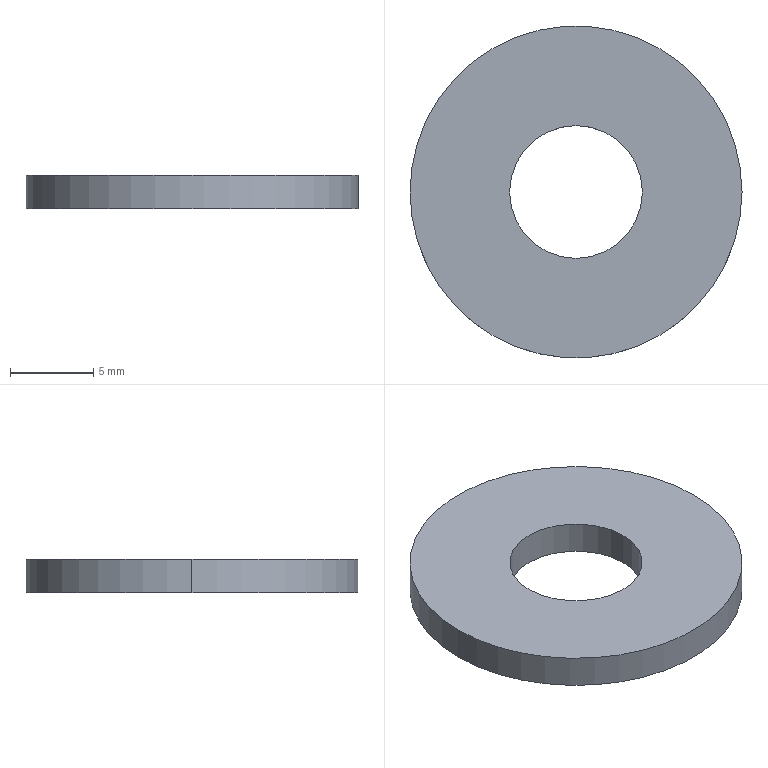Part | SolidWorks | features Extrusion 1 | 1 solid | 6 faces | box 20 x 20 x 2 mm | volume 527.788 mm3 | cylinder 4 | plane 2 | commonest cylinder face diameters 8 x2 20 x2
STEP:
#1=CARTESIAN_POINT('',(-4.,0.,2.));
#2=VERTEX_POINT('',#1);
#3=CARTESIAN_POINT('',(4.,0.,2.));
#4=VERTEX_POINT('',#3);
#5=CARTESIAN_POINT('',(0.,0.,2.));
#6=DIRECTION('',(0.,0.,1.));
#7=DIRECTION('',(1.,0.,0.));
#8=AXIS2_PLACEMENT_3D('',#5,#6,#7);
#9=CIRCLE('',#8,4.);
#10=EDGE_CURVE('',#2,#4,#9,.T.);
#11=ORIENTED_EDGE('',*,*,#10,.T.);
#12=CARTESIAN_POINT('',(4.,0.,0.));
#13=VERTEX_POINT('',#12);
#14=CARTESIAN_POINT('',(4.,0.,2.));
#15=DIRECTION('',(0.,0.,-1.));
#16=VECTOR('',#15,1000.);
#17=LINE('',#14,#16);
#18=EDGE_CURVE('',#4,#13,#17,.T.);
#19=ORIENTED_EDGE('',*,*,#18,.T.);
#20=CARTESIAN_POINT('',(-4.,0.,0.));
#21=VERTEX_POINT('',#20);
#22=CARTESIAN_POINT('',(0.,0.,0.));
#23=DIRECTION('',(0.,0.,1.));
#24=DIRECTION('',(1.,0.,0.));
#25=AXIS2_PLACEMENT_3D('',#22,#23,#24);
#26=CIRCLE('',#25,4.);
#27=EDGE_CURVE('',#21,#13,#26,.T.);
#28=ORIENTED_EDGE('',*,*,#27,.F.);
#29=CARTESIAN_POINT('',(-4.,0.,2.));
#30=DIRECTION('',(0.,0.,-1.));
#31=VECTOR('',#30,1000.);
#32=LINE('',#29,#31);
#33=EDGE_CURVE('',#2,#21,#32,.T.);
#34=ORIENTED_EDGE('',*,*,#33,.F.);
#35=EDGE_LOOP('',(#11,#19,#28,#34));
#36=FACE_OUTER_BOUND('',#35,.T.);
#37=CARTESIAN_POINT('',(0.,0.,2.));
#38=DIRECTION('',(0.,0.,-1.));
#39=DIRECTION('',(-1.,0.,0.));
#40=AXIS2_PLACEMENT_3D('',#37,#38,#39);
#41=CYLINDRICAL_SURFACE('',#40,4.);
#42=ADVANCED_FACE('',(#36),#41,.F.);
#43=CARTESIAN_POINT('',(10.,0.,2.));
#44=VERTEX_POINT('',#43);
#45=CARTESIAN_POINT('',(-10.,0.,2.));
#46=VERTEX_POINT('',#45);
#47=CARTESIAN_POINT('',(0.,0.,2.));
#48=DIRECTION('',(0.,0.,1.));
#49=DIRECTION('',(1.,0.,0.));
#50=AXIS2_PLACEMENT_3D('',#47,#48,#49);
#51=CIRCLE('',#50,10.);
#52=EDGE_CURVE('',#44,#46,#51,.T.);
#53=ORIENTED_EDGE('',*,*,#52,.F.);
#54=CARTESIAN_POINT('',(10.,0.,0.));
#55=VERTEX_POINT('',#54);
#56=CARTESIAN_POINT('',(10.,0.,2.));
#57=DIRECTION('',(0.,0.,-1.));
#58=VECTOR('',#57,1000.);
#59=LINE('',#56,#58);
#60=EDGE_CURVE('',#44,#55,#59,.T.);
#61=ORIENTED_EDGE('',*,*,#60,.T.);
#62=CARTESIAN_POINT('',(-10.,0.,0.));
#63=VERTEX_POINT('',#62);
#64=CARTESIAN_POINT('',(0.,0.,0.));
#65=DIRECTION('',(0.,0.,1.));
#66=DIRECTION('',(1.,0.,0.));
#67=AXIS2_PLACEMENT_3D('',#64,#65,#66);
#68=CIRCLE('',#67,10.);
#69=EDGE_CURVE('',#55,#63,#68,.T.);
#70=ORIENTED_EDGE('',*,*,#69,.T.);
#71=CARTESIAN_POINT('',(-10.,0.,2.));
#72=DIRECTION('',(0.,0.,-1.));
#73=VECTOR('',#72,1000.);
#74=LINE('',#71,#73);
#75=EDGE_CURVE('',#46,#63,#74,.T.);
#76=ORIENTED_EDGE('',*,*,#75,.F.);
#77=EDGE_LOOP('',(#53,#61,#70,#76));
#78=FACE_OUTER_BOUND('',#77,.T.);
#79=CARTESIAN_POINT('',(0.,0.,2.));
#80=DIRECTION('',(0.,0.,-1.));
#81=DIRECTION('',(-1.,0.,0.));
#82=AXIS2_PLACEMENT_3D('',#79,#80,#81);
#83=CYLINDRICAL_SURFACE('',#82,10.);
#84=ADVANCED_FACE('',(#78),#83,.T.);
#85=CARTESIAN_POINT('',(0.,0.,2.));
#86=DIRECTION('',(0.,0.,1.));
#87=DIRECTION('',(1.,0.,0.));
#88=AXIS2_PLACEMENT_3D('',#85,#86,#87);
#89=CIRCLE('',#88,10.);
#90=EDGE_CURVE('',#46,#44,#89,.T.);
#91=ORIENTED_EDGE('',*,*,#90,.T.);
#92=ORIENTED_EDGE('',*,*,#52,.T.);
#93=EDGE_LOOP('',(#91,#92));
#94=FACE_OUTER_BOUND('',#93,.T.);
#95=ORIENTED_EDGE('',*,*,#10,.F.);
#96=CARTESIAN_POINT('',(0.,0.,2.));
#97=DIRECTION('',(0.,0.,1.));
#98=DIRECTION('',(1.,0.,0.));
#99=AXIS2_PLACEMENT_3D('',#96,#97,#98);
#100=CIRCLE('',#99,4.);
#101=EDGE_CURVE('',#4,#2,#100,.T.);
#102=ORIENTED_EDGE('',*,*,#101,.F.);
#103=EDGE_LOOP('',(#95,#102));
#104=FACE_BOUND('',#103,.T.);
#105=CARTESIAN_POINT('',(0.,0.,2.));
#106=DIRECTION('',(0.,0.,1.));
#107=DIRECTION('',(1.,0.,0.));
#108=AXIS2_PLACEMENT_3D('',#105,#106,#107);
#109=PLANE('',#108);
#110=ADVANCED_FACE('',(#94,#104),#109,.T.);
#111=CARTESIAN_POINT('',(0.,0.,0.));
#112=DIRECTION('',(0.,0.,1.));
#113=DIRECTION('',(1.,0.,0.));
#114=AXIS2_PLACEMENT_3D('',#111,#112,#113);
#115=CIRCLE('',#114,10.);
#116=EDGE_CURVE('',#63,#55,#115,.T.);
#117=ORIENTED_EDGE('',*,*,#116,.F.);
#118=ORIENTED_EDGE('',*,*,#69,.F.);
#119=EDGE_LOOP('',(#117,#118));
#120=FACE_OUTER_BOUND('',#119,.T.);
#121=ORIENTED_EDGE('',*,*,#27,.T.);
#122=CARTESIAN_POINT('',(0.,0.,0.));
#123=DIRECTION('',(0.,0.,1.));
#124=DIRECTION('',(1.,0.,0.));
#125=AXIS2_PLACEMENT_3D('',#122,#123,#124);
#126=CIRCLE('',#125,4.);
#127=EDGE_CURVE('',#13,#21,#126,.T.);
#128=ORIENTED_EDGE('',*,*,#127,.T.);
#129=EDGE_LOOP('',(#121,#128));
#130=FACE_BOUND('',#129,.T.);
#131=CARTESIAN_POINT('',(0.,0.,0.));
#132=DIRECTION('',(0.,0.,1.));
#133=DIRECTION('',(1.,0.,0.));
#134=AXIS2_PLACEMENT_3D('',#131,#132,#133);
#135=PLANE('',#134);
#136=ADVANCED_FACE('',(#120,#130),#135,.F.);
#137=ORIENTED_EDGE('',*,*,#60,.F.);
#138=ORIENTED_EDGE('',*,*,#90,.F.);
#139=ORIENTED_EDGE('',*,*,#75,.T.);
#140=ORIENTED_EDGE('',*,*,#116,.T.);
#141=EDGE_LOOP('',(#137,#138,#139,#140));
#142=FACE_OUTER_BOUND('',#141,.T.);
#143=CARTESIAN_POINT('',(0.,0.,2.));
#144=DIRECTION('',(0.,0.,-1.));
#145=DIRECTION('',(-1.,0.,0.));
#146=AXIS2_PLACEMENT_3D('',#143,#144,#145);
#147=CYLINDRICAL_SURFACE('',#146,10.);
#148=ADVANCED_FACE('',(#142),#147,.T.);
#149=ORIENTED_EDGE('',*,*,#18,.F.);
#150=ORIENTED_EDGE('',*,*,#101,.T.);
#151=ORIENTED_EDGE('',*,*,#33,.T.);
#152=ORIENTED_EDGE('',*,*,#127,.F.);
#153=EDGE_LOOP('',(#149,#150,#151,#152));
#154=FACE_OUTER_BOUND('',#153,.T.);
#155=CARTESIAN_POINT('',(0.,0.,2.));
#156=DIRECTION('',(0.,0.,-1.));
#157=DIRECTION('',(-1.,0.,0.));
#158=AXIS2_PLACEMENT_3D('',#155,#156,#157);
#159=CYLINDRICAL_SURFACE('',#158,4.);
#160=ADVANCED_FACE('',(#154),#159,.F.);
#161=CLOSED_SHELL('',(#42,#84,#110,#136,#148,#160));
#162=MANIFOLD_SOLID_BREP('',#161);
#163=CARTESIAN_POINT('',(0.,0.,0.));
#164=DIRECTION('',(0.,0.,1.));
#165=DIRECTION('',(1.,0.,0.));
#166=AXIS2_PLACEMENT_3D('',#163,#164,#165);
#167=(LENGTH_UNIT()NAMED_UNIT(*)SI_UNIT(.MILLI.,.METRE.));
#168=UNCERTAINTY_MEASURE_WITH_UNIT(LENGTH_MEASURE(0.00001),#167,'','');
#169=(NAMED_UNIT(*)PLANE_ANGLE_UNIT()SI_UNIT($,.RADIAN.));
#170=(NAMED_UNIT(*)SI_UNIT($,.STERADIAN.)SOLID_ANGLE_UNIT());
#171=(GEOMETRIC_REPRESENTATION_CONTEXT(3)GLOBAL_UNCERTAINTY_ASSIGNED_CONTEXT((#168))GLOBAL_UNIT_ASSIGNED_CONTEXT((#167,#169,#170))REPRESENTATION_CONTEXT('',''));
#172=ADVANCED_BREP_SHAPE_REPRESENTATION('',(#162,#166),#171);